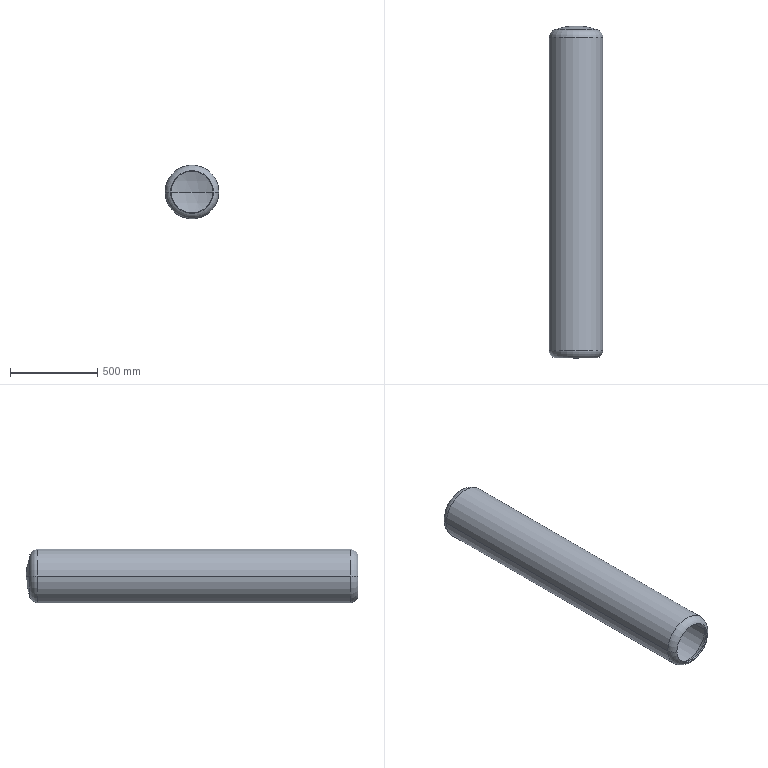Part | SolidWorks | features Revolution 1, Shell 1 | 1 solid | 18 faces | box 310 x 1908 x 310 mm | volume 14769515 mm3 | torus 8 | cylinder 4 | sphere 4 | cone 2 | commonest cylinder face diameters 294 x2 310 x2
STEP:
#1=CARTESIAN_POINT('',(119.998,-935.12,0.));
#2=VERTEX_POINT('',#1);
#3=CARTESIAN_POINT('',(-119.998,-935.12,0.));
#4=VERTEX_POINT('',#3);
#5=CARTESIAN_POINT('',(0.,-935.12,0.));
#6=DIRECTION('',(0.,1.,0.));
#7=DIRECTION('',(-1.,0.,0.));
#8=AXIS2_PLACEMENT_3D('',#5,#6,#7);
#9=CIRCLE('',#8,119.998);
#10=EDGE_CURVE('',#2,#4,#9,.T.);
#11=ORIENTED_EDGE('',*,*,#10,.F.);
#12=CARTESIAN_POINT('',(147.,-899.651,0.));
#13=VERTEX_POINT('',#12);
#14=CARTESIAN_POINT('',(105.175,-895.823,0.));
#15=DIRECTION('',(0.,0.,1.));
#16=DIRECTION('',(1.,0.,0.));
#17=AXIS2_PLACEMENT_3D('',#14,#15,#16);
#18=CIRCLE('',#17,42.);
#19=EDGE_CURVE('',#2,#13,#18,.T.);
#20=ORIENTED_EDGE('',*,*,#19,.T.);
#21=CARTESIAN_POINT('',(-147.,-899.651,0.));
#22=VERTEX_POINT('',#21);
#23=CARTESIAN_POINT('',(0.,-899.651,0.));
#24=DIRECTION('',(0.,1.,0.));
#25=DIRECTION('',(-1.,0.,0.));
#26=AXIS2_PLACEMENT_3D('',#23,#24,#25);
#27=CIRCLE('',#26,147.);
#28=EDGE_CURVE('',#13,#22,#27,.T.);
#29=ORIENTED_EDGE('',*,*,#28,.T.);
#30=CARTESIAN_POINT('',(-105.175,-895.823,0.));
#31=DIRECTION('',(0.,0.,-1.));
#32=DIRECTION('',(-1.,0.,0.));
#33=AXIS2_PLACEMENT_3D('',#30,#31,#32);
#34=CIRCLE('',#33,42.);
#35=EDGE_CURVE('',#4,#22,#34,.T.);
#36=ORIENTED_EDGE('',*,*,#35,.F.);
#37=EDGE_LOOP('',(#11,#20,#29,#36));
#38=FACE_OUTER_BOUND('',#37,.T.);
#39=CARTESIAN_POINT('',(0.,-895.823,0.));
#40=DIRECTION('',(0.,1.,0.));
#41=DIRECTION('',(-1.,0.,0.));
#42=AXIS2_PLACEMENT_3D('',#39,#40,#41);
#43=TOROIDAL_SURFACE('',#42,105.175,42.);
#44=ADVANCED_FACE('',(#38),#43,.F.);
#45=ORIENTED_EDGE('',*,*,#28,.F.);
#46=CARTESIAN_POINT('',(147.,899.651,0.));
#47=VERTEX_POINT('',#46);
#48=CARTESIAN_POINT('',(147.,965.,0.));
#49=DIRECTION('',(0.,1.,0.));
#50=VECTOR('',#49,1000.);
#51=LINE('',#48,#50);
#52=EDGE_CURVE('',#13,#47,#51,.T.);
#53=ORIENTED_EDGE('',*,*,#52,.T.);
#54=CARTESIAN_POINT('',(-147.,899.651,0.));
#55=VERTEX_POINT('',#54);
#56=CARTESIAN_POINT('',(0.,899.651,0.));
#57=DIRECTION('',(0.,1.,0.));
#58=DIRECTION('',(1.,0.,0.));
#59=AXIS2_PLACEMENT_3D('',#56,#57,#58);
#60=CIRCLE('',#59,147.);
#61=EDGE_CURVE('',#47,#55,#60,.T.);
#62=ORIENTED_EDGE('',*,*,#61,.T.);
#63=CARTESIAN_POINT('',(-147.,965.,0.));
#64=DIRECTION('',(0.,1.,0.));
#65=VECTOR('',#64,1000.);
#66=LINE('',#63,#65);
#67=EDGE_CURVE('',#22,#55,#66,.T.);
#68=ORIENTED_EDGE('',*,*,#67,.F.);
#69=EDGE_LOOP('',(#45,#53,#62,#68));
#70=FACE_OUTER_BOUND('',#69,.T.);
#71=CARTESIAN_POINT('',(0.,965.,0.));
#72=DIRECTION('',(0.,1.,0.));
#73=DIRECTION('',(-1.,0.,0.));
#74=AXIS2_PLACEMENT_3D('',#71,#72,#73);
#75=CYLINDRICAL_SURFACE('',#74,147.);
#76=ADVANCED_FACE('',(#70),#75,.F.);
#77=ORIENTED_EDGE('',*,*,#61,.F.);
#78=CARTESIAN_POINT('',(119.998,935.12,0.));
#79=VERTEX_POINT('',#78);
#80=CARTESIAN_POINT('',(105.175,895.823,0.));
#81=DIRECTION('',(0.,0.,1.));
#82=DIRECTION('',(1.,0.,0.));
#83=AXIS2_PLACEMENT_3D('',#80,#81,#82);
#84=CIRCLE('',#83,42.);
#85=EDGE_CURVE('',#47,#79,#84,.T.);
#86=ORIENTED_EDGE('',*,*,#85,.T.);
#87=CARTESIAN_POINT('',(-119.998,935.12,0.));
#88=VERTEX_POINT('',#87);
#89=CARTESIAN_POINT('',(0.,935.12,0.));
#90=DIRECTION('',(0.,1.,0.));
#91=DIRECTION('',(-1.,0.,0.));
#92=AXIS2_PLACEMENT_3D('',#89,#90,#91);
#93=CIRCLE('',#92,119.998);
#94=EDGE_CURVE('',#79,#88,#93,.T.);
#95=ORIENTED_EDGE('',*,*,#94,.T.);
#96=CARTESIAN_POINT('',(-105.175,895.823,0.));
#97=DIRECTION('',(0.,0.,-1.));
#98=DIRECTION('',(-1.,0.,0.));
#99=AXIS2_PLACEMENT_3D('',#96,#97,#98);
#100=CIRCLE('',#99,42.);
#101=EDGE_CURVE('',#55,#88,#100,.T.);
#102=ORIENTED_EDGE('',*,*,#101,.F.);
#103=EDGE_LOOP('',(#77,#86,#95,#102));
#104=FACE_OUTER_BOUND('',#103,.T.);
#105=CARTESIAN_POINT('',(0.,895.823,0.));
#106=DIRECTION('',(0.,1.,0.));
#107=DIRECTION('',(-1.,0.,0.));
#108=AXIS2_PLACEMENT_3D('',#105,#106,#107);
#109=TOROIDAL_SURFACE('',#108,105.175,42.);
#110=ADVANCED_FACE('',(#104),#109,.F.);
#111=CARTESIAN_POINT('',(0.,935.12,0.));
#112=DIRECTION('',(0.,1.,0.));
#113=DIRECTION('',(-1.,0.,0.));
#114=AXIS2_PLACEMENT_3D('',#111,#112,#113);
#115=CIRCLE('',#114,119.998);
#116=EDGE_CURVE('',#88,#79,#115,.T.);
#117=ORIENTED_EDGE('',*,*,#116,.F.);
#118=CARTESIAN_POINT('',(0.,957.,0.));
#119=VERTEX_POINT('',#118);
#120=CARTESIAN_POINT('',(0.,617.,0.));
#121=DIRECTION('',(0.,0.,-1.));
#122=DIRECTION('',(-1.,0.,0.));
#123=AXIS2_PLACEMENT_3D('',#120,#121,#122);
#124=CIRCLE('',#123,340.);
#125=EDGE_CURVE('',#88,#119,#124,.T.);
#126=ORIENTED_EDGE('',*,*,#125,.T.);
#127=CARTESIAN_POINT('',(0.,617.,0.));
#128=DIRECTION('',(0.,0.,1.));
#129=DIRECTION('',(1.,0.,0.));
#130=AXIS2_PLACEMENT_3D('',#127,#128,#129);
#131=CIRCLE('',#130,340.);
#132=EDGE_CURVE('',#79,#119,#131,.T.);
#133=ORIENTED_EDGE('',*,*,#132,.F.);
#134=EDGE_LOOP('',(#117,#126,#133));
#135=FACE_OUTER_BOUND('',#134,.T.);
#136=CARTESIAN_POINT('',(0.,617.,0.));
#137=DIRECTION('',(0.,0.,-1.));
#138=DIRECTION('',(1.,0.,0.));
#139=AXIS2_PLACEMENT_3D('',#136,#137,#138);
#140=SPHERICAL_SURFACE('',#139,340.);
#141=ADVANCED_FACE('',(#135),#140,.F.);
#142=ORIENTED_EDGE('',*,*,#10,.T.);
#143=CARTESIAN_POINT('',(-122.822,-942.605,0.));
#144=VERTEX_POINT('',#143);
#145=CARTESIAN_POINT('',(-122.822,-942.605,0.));
#146=DIRECTION('',(-0.3529,-0.9356,0.));
#147=VECTOR('',#146,1000.);
#148=LINE('',#145,#147);
#149=EDGE_CURVE('',#4,#144,#148,.T.);
#150=ORIENTED_EDGE('',*,*,#149,.T.);
#151=CARTESIAN_POINT('',(122.822,-942.605,0.));
#152=VERTEX_POINT('',#151);
#153=CARTESIAN_POINT('',(0.,-942.605,0.));
#154=DIRECTION('',(0.,1.,0.));
#155=DIRECTION('',(-1.,0.,0.));
#156=AXIS2_PLACEMENT_3D('',#153,#154,#155);
#157=CIRCLE('',#156,122.822);
#158=EDGE_CURVE('',#152,#144,#157,.T.);
#159=ORIENTED_EDGE('',*,*,#158,.F.);
#160=CARTESIAN_POINT('',(122.822,-942.605,0.));
#161=DIRECTION('',(0.3529,-0.9356,0.));
#162=VECTOR('',#161,1000.);
#163=LINE('',#160,#162);
#164=EDGE_CURVE('',#2,#152,#163,.T.);
#165=ORIENTED_EDGE('',*,*,#164,.F.);
#166=EDGE_LOOP('',(#142,#150,#159,#165));
#167=FACE_OUTER_BOUND('',#166,.T.);
#168=CARTESIAN_POINT('',(0.,-942.605,0.));
#169=DIRECTION('',(0.,-1.,0.));
#170=DIRECTION('',(1.,0.,0.));
#171=AXIS2_PLACEMENT_3D('',#168,#169,#170);
#172=CONICAL_SURFACE('',#171,122.822,0.3607);
#173=ADVANCED_FACE('',(#167),#172,.F.);
#174=CARTESIAN_POINT('',(0.,-942.605,0.));
#175=DIRECTION('',(0.,1.,0.));
#176=DIRECTION('',(-1.,0.,0.));
#177=AXIS2_PLACEMENT_3D('',#174,#175,#176);
#178=CIRCLE('',#177,122.822);
#179=EDGE_CURVE('',#144,#152,#178,.T.);
#180=ORIENTED_EDGE('',*,*,#179,.T.);
#181=CARTESIAN_POINT('',(155.,-900.,0.));
#182=VERTEX_POINT('',#181);
#183=CARTESIAN_POINT('',(105.175,-895.823,0.));
#184=DIRECTION('',(0.,0.,1.));
#185=DIRECTION('',(1.,0.,0.));
#186=AXIS2_PLACEMENT_3D('',#183,#184,#185);
#187=CIRCLE('',#186,50.);
#188=EDGE_CURVE('',#152,#182,#187,.T.);
#189=ORIENTED_EDGE('',*,*,#188,.T.);
#190=CARTESIAN_POINT('',(-155.,-900.,0.));
#191=VERTEX_POINT('',#190);
#192=CARTESIAN_POINT('',(0.,-900.,0.));
#193=DIRECTION('',(0.,1.,0.));
#194=DIRECTION('',(-1.,0.,0.));
#195=AXIS2_PLACEMENT_3D('',#192,#193,#194);
#196=CIRCLE('',#195,155.);
#197=EDGE_CURVE('',#191,#182,#196,.T.);
#198=ORIENTED_EDGE('',*,*,#197,.F.);
#199=CARTESIAN_POINT('',(-105.175,-895.823,0.));
#200=DIRECTION('',(0.,0.,-1.));
#201=DIRECTION('',(-1.,0.,0.));
#202=AXIS2_PLACEMENT_3D('',#199,#200,#201);
#203=CIRCLE('',#202,50.);
#204=EDGE_CURVE('',#144,#191,#203,.T.);
#205=ORIENTED_EDGE('',*,*,#204,.F.);
#206=EDGE_LOOP('',(#180,#189,#198,#205));
#207=FACE_OUTER_BOUND('',#206,.T.);
#208=CARTESIAN_POINT('',(0.,-895.823,0.));
#209=DIRECTION('',(0.,1.,0.));
#210=DIRECTION('',(-1.,0.,0.));
#211=AXIS2_PLACEMENT_3D('',#208,#209,#210);
#212=TOROIDAL_SURFACE('',#211,105.175,50.);
#213=ADVANCED_FACE('',(#207),#212,.T.);
#214=ORIENTED_EDGE('',*,*,#197,.T.);
#215=CARTESIAN_POINT('',(155.,900.,0.));
#216=VERTEX_POINT('',#215);
#217=CARTESIAN_POINT('',(155.,965.,0.));
#218=DIRECTION('',(0.,1.,0.));
#219=VECTOR('',#218,1000.);
#220=LINE('',#217,#219);
#221=EDGE_CURVE('',#182,#216,#220,.T.);
#222=ORIENTED_EDGE('',*,*,#221,.T.);
#223=CARTESIAN_POINT('',(-155.,900.,0.));
#224=VERTEX_POINT('',#223);
#225=CARTESIAN_POINT('',(0.,900.,0.));
#226=DIRECTION('',(0.,1.,0.));
#227=DIRECTION('',(-1.,0.,0.));
#228=AXIS2_PLACEMENT_3D('',#225,#226,#227);
#229=CIRCLE('',#228,155.);
#230=EDGE_CURVE('',#224,#216,#229,.T.);
#231=ORIENTED_EDGE('',*,*,#230,.F.);
#232=CARTESIAN_POINT('',(-155.,965.,0.));
#233=DIRECTION('',(0.,1.,0.));
#234=VECTOR('',#233,1000.);
#235=LINE('',#232,#234);
#236=EDGE_CURVE('',#191,#224,#235,.T.);
#237=ORIENTED_EDGE('',*,*,#236,.F.);
#238=EDGE_LOOP('',(#214,#222,#231,#237));
#239=FACE_OUTER_BOUND('',#238,.T.);
#240=CARTESIAN_POINT('',(0.,965.,0.));
#241=DIRECTION('',(0.,1.,0.));
#242=DIRECTION('',(-1.,0.,0.));
#243=AXIS2_PLACEMENT_3D('',#240,#241,#242);
#244=CYLINDRICAL_SURFACE('',#243,155.);
#245=ADVANCED_FACE('',(#239),#244,.T.);
#246=ORIENTED_EDGE('',*,*,#230,.T.);
#247=CARTESIAN_POINT('',(122.822,942.605,0.));
#248=VERTEX_POINT('',#247);
#249=CARTESIAN_POINT('',(105.175,895.823,0.));
#250=DIRECTION('',(0.,0.,1.));
#251=DIRECTION('',(1.,0.,0.));
#252=AXIS2_PLACEMENT_3D('',#249,#250,#251);
#253=CIRCLE('',#252,50.);
#254=EDGE_CURVE('',#216,#248,#253,.T.);
#255=ORIENTED_EDGE('',*,*,#254,.T.);
#256=CARTESIAN_POINT('',(-122.822,942.605,0.));
#257=VERTEX_POINT('',#256);
#258=CARTESIAN_POINT('',(0.,942.605,0.));
#259=DIRECTION('',(0.,1.,0.));
#260=DIRECTION('',(-1.,0.,0.));
#261=AXIS2_PLACEMENT_3D('',#258,#259,#260);
#262=CIRCLE('',#261,122.822);
#263=EDGE_CURVE('',#257,#248,#262,.T.);
#264=ORIENTED_EDGE('',*,*,#263,.F.);
#265=CARTESIAN_POINT('',(-105.175,895.823,0.));
#266=DIRECTION('',(0.,0.,-1.));
#267=DIRECTION('',(-1.,0.,0.));
#268=AXIS2_PLACEMENT_3D('',#265,#266,#267);
#269=CIRCLE('',#268,50.);
#270=EDGE_CURVE('',#224,#257,#269,.T.);
#271=ORIENTED_EDGE('',*,*,#270,.F.);
#272=EDGE_LOOP('',(#246,#255,#264,#271));
#273=FACE_OUTER_BOUND('',#272,.T.);
#274=CARTESIAN_POINT('',(0.,895.823,0.));
#275=DIRECTION('',(0.,1.,0.));
#276=DIRECTION('',(-1.,0.,0.));
#277=AXIS2_PLACEMENT_3D('',#274,#275,#276);
#278=TOROIDAL_SURFACE('',#277,105.175,50.);
#279=ADVANCED_FACE('',(#273),#278,.T.);
#280=CARTESIAN_POINT('',(0.,942.605,0.));
#281=DIRECTION('',(0.,1.,0.));
#282=DIRECTION('',(-1.,0.,0.));
#283=AXIS2_PLACEMENT_3D('',#280,#281,#282);
#284=CIRCLE('',#283,122.822);
#285=EDGE_CURVE('',#248,#257,#284,.T.);
#286=ORIENTED_EDGE('',*,*,#285,.T.);
#287=CARTESIAN_POINT('',(0.,965.,0.));
#288=VERTEX_POINT('',#287);
#289=CARTESIAN_POINT('',(0.,617.,0.));
#290=DIRECTION('',(0.,0.,-1.));
#291=DIRECTION('',(-1.,0.,0.));
#292=AXIS2_PLACEMENT_3D('',#289,#290,#291);
#293=CIRCLE('',#292,348.);
#294=EDGE_CURVE('',#257,#288,#293,.T.);
#295=ORIENTED_EDGE('',*,*,#294,.T.);
#296=CARTESIAN_POINT('',(0.,617.,0.));
#297=DIRECTION('',(0.,0.,1.));
#298=DIRECTION('',(1.,0.,0.));
#299=AXIS2_PLACEMENT_3D('',#296,#297,#298);
#300=CIRCLE('',#299,348.);
#301=EDGE_CURVE('',#248,#288,#300,.T.);
#302=ORIENTED_EDGE('',*,*,#301,.F.);
#303=EDGE_LOOP('',(#286,#295,#302));
#304=FACE_OUTER_BOUND('',#303,.T.);
#305=CARTESIAN_POINT('',(0.,617.,0.));
#306=DIRECTION('',(0.,0.,-1.));
#307=DIRECTION('',(1.,0.,0.));
#308=AXIS2_PLACEMENT_3D('',#305,#306,#307);
#309=SPHERICAL_SURFACE('',#308,348.);
#310=ADVANCED_FACE('',(#304),#309,.T.);
#311=ORIENTED_EDGE('',*,*,#294,.F.);
#312=ORIENTED_EDGE('',*,*,#263,.T.);
#313=ORIENTED_EDGE('',*,*,#301,.T.);
#314=EDGE_LOOP('',(#311,#312,#313));
#315=FACE_OUTER_BOUND('',#314,.T.);
#316=CARTESIAN_POINT('',(0.,617.,0.));
#317=DIRECTION('',(0.,0.,-1.));
#318=DIRECTION('',(1.,0.,0.));
#319=AXIS2_PLACEMENT_3D('',#316,#317,#318);
#320=SPHERICAL_SURFACE('',#319,348.);
#321=ADVANCED_FACE('',(#315),#320,.T.);
#322=ORIENTED_EDGE('',*,*,#254,.F.);
#323=CARTESIAN_POINT('',(0.,900.,0.));
#324=DIRECTION('',(0.,1.,0.));
#325=DIRECTION('',(-1.,0.,0.));
#326=AXIS2_PLACEMENT_3D('',#323,#324,#325);
#327=CIRCLE('',#326,155.);
#328=EDGE_CURVE('',#216,#224,#327,.T.);
#329=ORIENTED_EDGE('',*,*,#328,.T.);
#330=ORIENTED_EDGE('',*,*,#270,.T.);
#331=ORIENTED_EDGE('',*,*,#285,.F.);
#332=EDGE_LOOP('',(#322,#329,#330,#331));
#333=FACE_OUTER_BOUND('',#332,.T.);
#334=CARTESIAN_POINT('',(0.,895.823,0.));
#335=DIRECTION('',(0.,1.,0.));
#336=DIRECTION('',(-1.,0.,0.));
#337=AXIS2_PLACEMENT_3D('',#334,#335,#336);
#338=TOROIDAL_SURFACE('',#337,105.175,50.);
#339=ADVANCED_FACE('',(#333),#338,.T.);
#340=ORIENTED_EDGE('',*,*,#221,.F.);
#341=CARTESIAN_POINT('',(0.,-900.,0.));
#342=DIRECTION('',(0.,1.,0.));
#343=DIRECTION('',(-1.,0.,0.));
#344=AXIS2_PLACEMENT_3D('',#341,#342,#343);
#345=CIRCLE('',#344,155.);
#346=EDGE_CURVE('',#182,#191,#345,.T.);
#347=ORIENTED_EDGE('',*,*,#346,.T.);
#348=ORIENTED_EDGE('',*,*,#236,.T.);
#349=ORIENTED_EDGE('',*,*,#328,.F.);
#350=EDGE_LOOP('',(#340,#347,#348,#349));
#351=FACE_OUTER_BOUND('',#350,.T.);
#352=CARTESIAN_POINT('',(0.,965.,0.));
#353=DIRECTION('',(0.,1.,0.));
#354=DIRECTION('',(-1.,0.,0.));
#355=AXIS2_PLACEMENT_3D('',#352,#353,#354);
#356=CYLINDRICAL_SURFACE('',#355,155.);
#357=ADVANCED_FACE('',(#351),#356,.T.);
#358=ORIENTED_EDGE('',*,*,#188,.F.);
#359=ORIENTED_EDGE('',*,*,#158,.T.);
#360=ORIENTED_EDGE('',*,*,#204,.T.);
#361=ORIENTED_EDGE('',*,*,#346,.F.);
#362=EDGE_LOOP('',(#358,#359,#360,#361));
#363=FACE_OUTER_BOUND('',#362,.T.);
#364=CARTESIAN_POINT('',(0.,-895.823,0.));
#365=DIRECTION('',(0.,1.,0.));
#366=DIRECTION('',(-1.,0.,0.));
#367=AXIS2_PLACEMENT_3D('',#364,#365,#366);
#368=TOROIDAL_SURFACE('',#367,105.175,50.);
#369=ADVANCED_FACE('',(#363),#368,.T.);
#370=ORIENTED_EDGE('',*,*,#149,.F.);
#371=CARTESIAN_POINT('',(0.,-935.12,0.));
#372=DIRECTION('',(0.,1.,0.));
#373=DIRECTION('',(-1.,0.,0.));
#374=AXIS2_PLACEMENT_3D('',#371,#372,#373);
#375=CIRCLE('',#374,119.998);
#376=EDGE_CURVE('',#4,#2,#375,.T.);
#377=ORIENTED_EDGE('',*,*,#376,.T.);
#378=ORIENTED_EDGE('',*,*,#164,.T.);
#379=ORIENTED_EDGE('',*,*,#179,.F.);
#380=EDGE_LOOP('',(#370,#377,#378,#379));
#381=FACE_OUTER_BOUND('',#380,.T.);
#382=CARTESIAN_POINT('',(0.,-942.605,0.));
#383=DIRECTION('',(0.,-1.,0.));
#384=DIRECTION('',(1.,0.,0.));
#385=AXIS2_PLACEMENT_3D('',#382,#383,#384);
#386=CONICAL_SURFACE('',#385,122.822,0.3607);
#387=ADVANCED_FACE('',(#381),#386,.F.);
#388=ORIENTED_EDGE('',*,*,#125,.F.);
#389=ORIENTED_EDGE('',*,*,#94,.F.);
#390=ORIENTED_EDGE('',*,*,#132,.T.);
#391=EDGE_LOOP('',(#388,#389,#390));
#392=FACE_OUTER_BOUND('',#391,.T.);
#393=CARTESIAN_POINT('',(0.,617.,0.));
#394=DIRECTION('',(0.,0.,-1.));
#395=DIRECTION('',(1.,0.,0.));
#396=AXIS2_PLACEMENT_3D('',#393,#394,#395);
#397=SPHERICAL_SURFACE('',#396,340.);
#398=ADVANCED_FACE('',(#392),#397,.F.);
#399=ORIENTED_EDGE('',*,*,#85,.F.);
#400=CARTESIAN_POINT('',(0.,899.651,0.));
#401=DIRECTION('',(0.,1.,0.));
#402=DIRECTION('',(1.,0.,0.));
#403=AXIS2_PLACEMENT_3D('',#400,#401,#402);
#404=CIRCLE('',#403,147.);
#405=EDGE_CURVE('',#55,#47,#404,.T.);
#406=ORIENTED_EDGE('',*,*,#405,.F.);
#407=ORIENTED_EDGE('',*,*,#101,.T.);
#408=ORIENTED_EDGE('',*,*,#116,.T.);
#409=EDGE_LOOP('',(#399,#406,#407,#408));
#410=FACE_OUTER_BOUND('',#409,.T.);
#411=CARTESIAN_POINT('',(0.,895.823,0.));
#412=DIRECTION('',(0.,1.,0.));
#413=DIRECTION('',(-1.,0.,0.));
#414=AXIS2_PLACEMENT_3D('',#411,#412,#413);
#415=TOROIDAL_SURFACE('',#414,105.175,42.);
#416=ADVANCED_FACE('',(#410),#415,.F.);
#417=ORIENTED_EDGE('',*,*,#52,.F.);
#418=CARTESIAN_POINT('',(0.,-899.651,0.));
#419=DIRECTION('',(0.,1.,0.));
#420=DIRECTION('',(-1.,0.,0.));
#421=AXIS2_PLACEMENT_3D('',#418,#419,#420);
#422=CIRCLE('',#421,147.);
#423=EDGE_CURVE('',#22,#13,#422,.T.);
#424=ORIENTED_EDGE('',*,*,#423,.F.);
#425=ORIENTED_EDGE('',*,*,#67,.T.);
#426=ORIENTED_EDGE('',*,*,#405,.T.);
#427=EDGE_LOOP('',(#417,#424,#425,#426));
#428=FACE_OUTER_BOUND('',#427,.T.);
#429=CARTESIAN_POINT('',(0.,965.,0.));
#430=DIRECTION('',(0.,1.,0.));
#431=DIRECTION('',(-1.,0.,0.));
#432=AXIS2_PLACEMENT_3D('',#429,#430,#431);
#433=CYLINDRICAL_SURFACE('',#432,147.);
#434=ADVANCED_FACE('',(#428),#433,.F.);
#435=ORIENTED_EDGE('',*,*,#19,.F.);
#436=ORIENTED_EDGE('',*,*,#376,.F.);
#437=ORIENTED_EDGE('',*,*,#35,.T.);
#438=ORIENTED_EDGE('',*,*,#423,.T.);
#439=EDGE_LOOP('',(#435,#436,#437,#438));
#440=FACE_OUTER_BOUND('',#439,.T.);
#441=CARTESIAN_POINT('',(0.,-895.823,0.));
#442=DIRECTION('',(0.,1.,0.));
#443=DIRECTION('',(-1.,0.,0.));
#444=AXIS2_PLACEMENT_3D('',#441,#442,#443);
#445=TOROIDAL_SURFACE('',#444,105.175,42.);
#446=ADVANCED_FACE('',(#440),#445,.F.);
#447=CLOSED_SHELL('',(#44,#76,#110,#141,#173,#213,#245,#279,#310,#321,#339,#357,#369,#387,#398,#416,#434,#446));
#448=MANIFOLD_SOLID_BREP('',#447);
#449=CARTESIAN_POINT('',(0.,0.,0.));
#450=DIRECTION('',(0.,0.,1.));
#451=DIRECTION('',(1.,0.,0.));
#452=AXIS2_PLACEMENT_3D('',#449,#450,#451);
#453=(LENGTH_UNIT()NAMED_UNIT(*)SI_UNIT(.MILLI.,.METRE.));
#454=UNCERTAINTY_MEASURE_WITH_UNIT(LENGTH_MEASURE(0.00001),#453,'','');
#455=(NAMED_UNIT(*)PLANE_ANGLE_UNIT()SI_UNIT($,.RADIAN.));
#456=(NAMED_UNIT(*)SI_UNIT($,.STERADIAN.)SOLID_ANGLE_UNIT());
#457=(GEOMETRIC_REPRESENTATION_CONTEXT(3)GLOBAL_UNCERTAINTY_ASSIGNED_CONTEXT((#454))GLOBAL_UNIT_ASSIGNED_CONTEXT((#453,#455,#456))REPRESENTATION_CONTEXT('',''));
#458=ADVANCED_BREP_SHAPE_REPRESENTATION('',(#448,#452),#457);